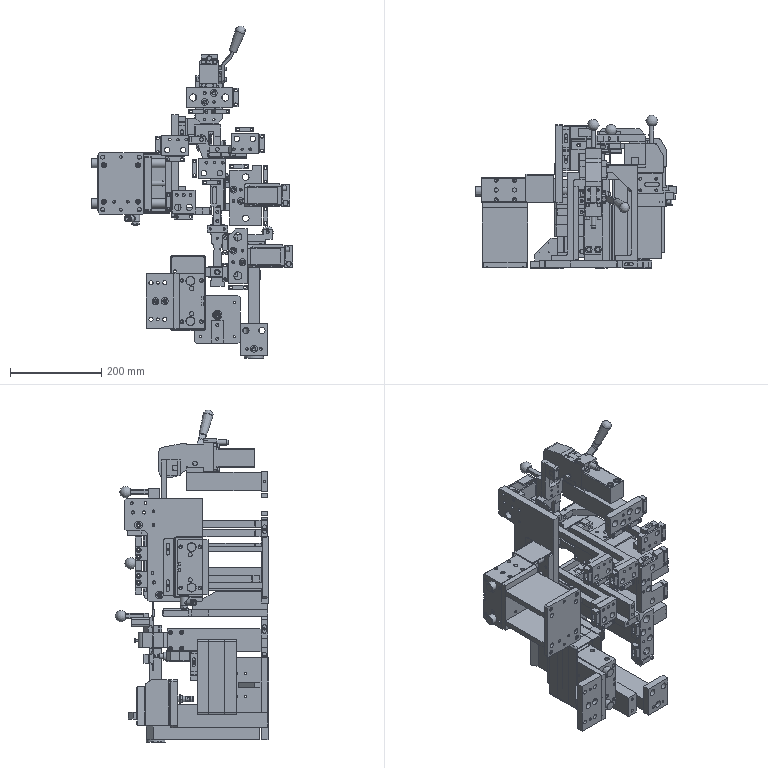Part | NX | features BREP 175 | 175 solids | 4272 faces | volume 8608160 mm3 | plane 2186 | cylinder 1514 | cone 512 | torus 32 | spline 18 | sphere 10 | commonest cylinder face diameters 6 x244 5 x129 8 x77 10 x68 9 x58 7 x57